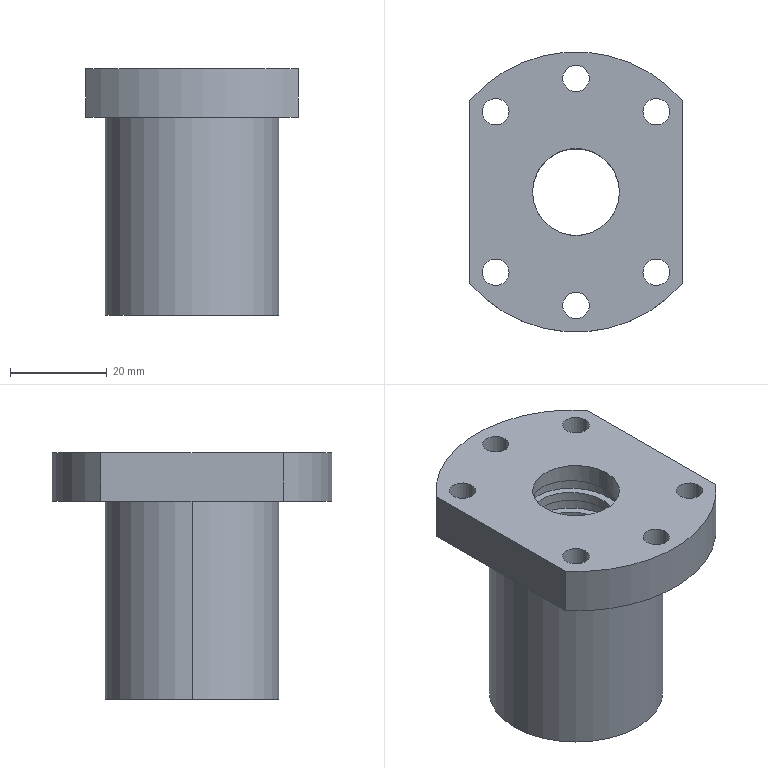Part | SolidWorks | features Extrusion 1, Helix 1, ICE 1, RefAxis 1, SweepCut 1 | 1 solid | 46 faces | box 44 x 58 x 51 mm | volume 47513 mm3 | cylinder 37 | plane 6 | spline 3 | commonest cylinder face diameters 18 x21 5.5 x12 36 x2 58 x2